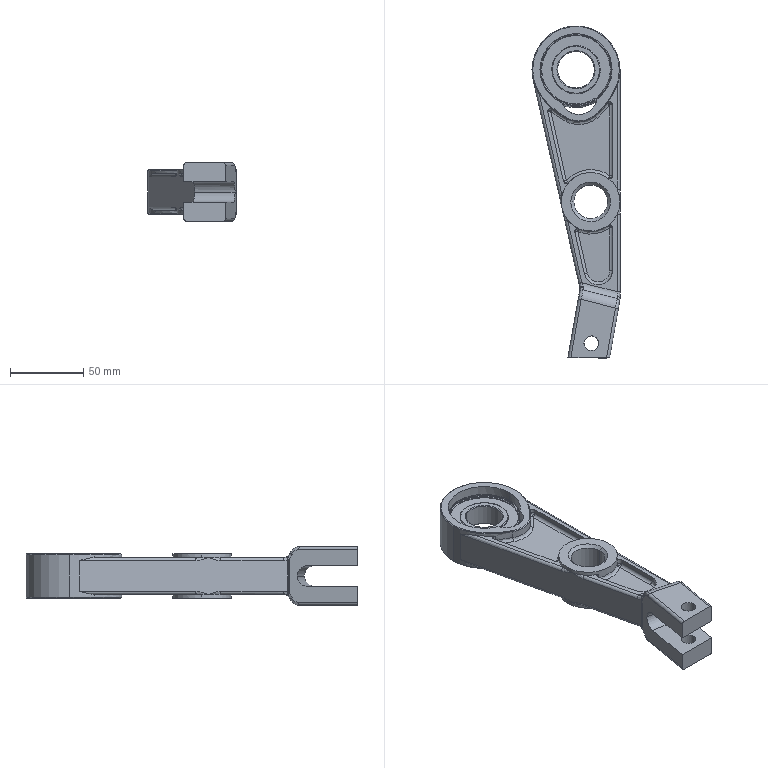Part | SolidWorks | features LayoutProfileFeature 1 | 2 solids | 216 faces | box 60 x 226.322 x 40 mm | volume 177077 mm3 | cylinder 81 | spline 78 | plane 38 | cone 19 | commonest cylinder face diameters 4 x36 10 x6 49.143 x6 14 x4 33 x4 40 x4